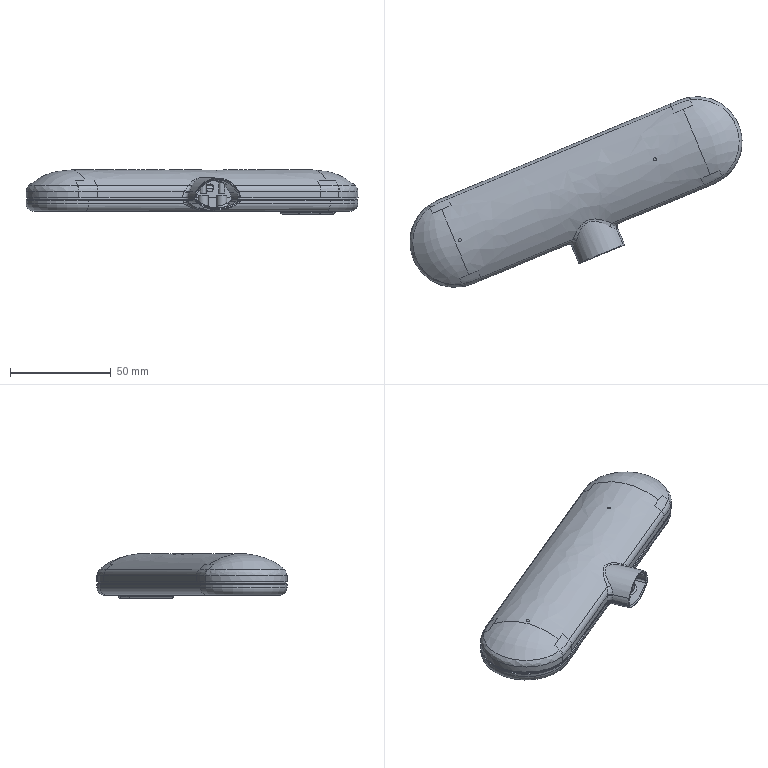Part | NX | features SKETCH 36, EXTRUDE 25, BLEND 21, DATUM_CSYS 15, HOLE PACKAGE 12, CBORE_HOLE 7, SIMPLE HOLE 7, DATUM_PLANE 6, SCALE 5, CHAMFER 3, EXTRACT_BODY 3, SEW 3, THRU_CURVE 3, THRU_CURVE_MESH 3, TRIM BODY 3, UNITE 3, BRIDGE_CURVE 2, CPROJ 2, Container 2, EXTRACT_FACE 2, Geometry Instance 2, SHELL 2, SWP104 2, TRIM_AND_EXTEND 2, DRAFT 1, SKIN 1, THICKEN_SHEET 1 | 4 solids | 373 faces | box 165.085 x 94.798 x 22.148 mm | volume 29752 mm3 | plane 124 | cylinder 119 | spline 88 | torus 26 | cone 10 | sphere 6 | commonest cylinder face diameters 2 x20 1 x18 1.5 x14 5 x14 4 x12 6 x5